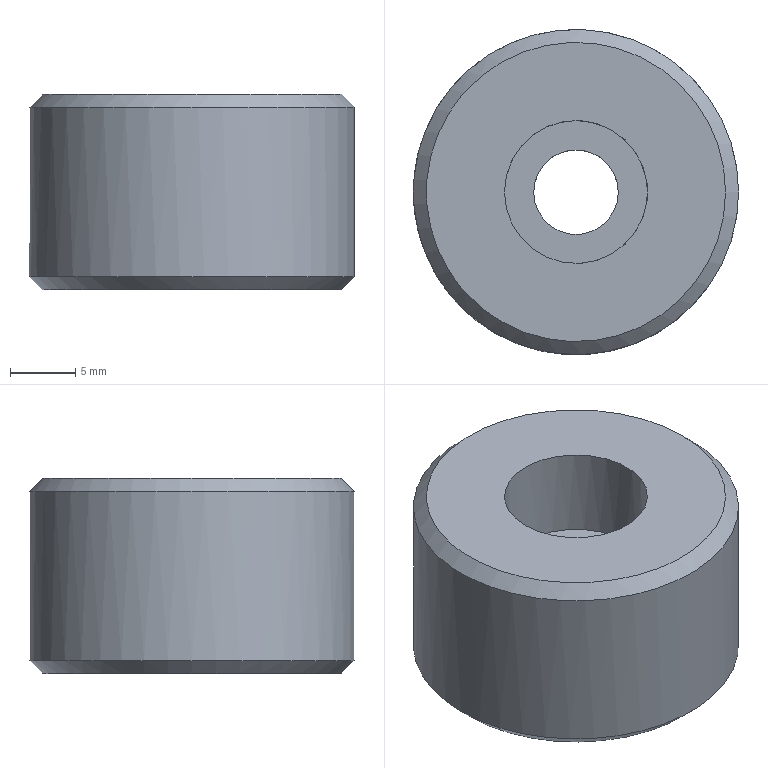Part | STEP file | lll_id122_x_t | 1 solid | 8 faces | box 25 x 25 x 15 mm | volume 6356 mm3 | plane 3 | cylinder 3 | cone 2 | commonest cylinder face diameters 6.5 x1 11 x1 25 x1
STEP:
#1=CARTESIAN_POINT('',(-28.5,-80.,-100.5));
#2=VERTEX_POINT('',#1);
#3=CARTESIAN_POINT('',(-40.,-80.,-100.5));
#4=DIRECTION('',(0.,0.,1.));
#5=DIRECTION('',(1.,0.,0.));
#6=AXIS2_PLACEMENT_3D('',#3,#4,#5);
#7=CIRCLE('',#6,11.5);
#8=EDGE_CURVE('',#2,#2,#7,.T.);
#9=ORIENTED_EDGE('',*,*,#8,.T.);
#10=EDGE_LOOP('',(#9));
#11=FACE_BOUND('',#10,.T.);
#12=CARTESIAN_POINT('',(-45.5,-80.,-100.5));
#13=VERTEX_POINT('',#12);
#14=CARTESIAN_POINT('',(-40.,-80.,-100.5));
#15=DIRECTION('',(0.,0.,-1.));
#16=DIRECTION('',(-1.,0.,0.));
#17=AXIS2_PLACEMENT_3D('',#14,#15,#16);
#18=CIRCLE('',#17,5.5);
#19=EDGE_CURVE('',#13,#13,#18,.T.);
#20=ORIENTED_EDGE('',*,*,#19,.T.);
#21=EDGE_LOOP('',(#20));
#22=FACE_BOUND('',#21,.T.);
#23=CARTESIAN_POINT('',(-40.,-80.,-100.5));
#24=DIRECTION('',(0.,0.,1.));
#25=DIRECTION('',(1.,0.,0.));
#26=AXIS2_PLACEMENT_3D('',#23,#24,#25);
#27=PLANE('',#26);
#28=ADVANCED_FACE('',(#11,#22),#27,.T.);
#29=CARTESIAN_POINT('',(-51.5,-80.,-115.5));
#30=VERTEX_POINT('',#29);
#31=CARTESIAN_POINT('',(-40.,-80.,-115.5));
#32=DIRECTION('',(0.,0.,-1.));
#33=DIRECTION('',(-1.,0.,0.));
#34=AXIS2_PLACEMENT_3D('',#31,#32,#33);
#35=CIRCLE('',#34,11.5);
#36=EDGE_CURVE('',#30,#30,#35,.T.);
#37=ORIENTED_EDGE('',*,*,#36,.T.);
#38=EDGE_LOOP('',(#37));
#39=FACE_BOUND('',#38,.T.);
#40=CARTESIAN_POINT('',(-36.75,-80.,-115.5));
#41=VERTEX_POINT('',#40);
#42=CARTESIAN_POINT('',(-40.,-80.,-115.5));
#43=DIRECTION('',(0.,0.,1.));
#44=DIRECTION('',(1.,0.,0.));
#45=AXIS2_PLACEMENT_3D('',#42,#43,#44);
#46=CIRCLE('',#45,3.25);
#47=EDGE_CURVE('',#41,#41,#46,.T.);
#48=ORIENTED_EDGE('',*,*,#47,.T.);
#49=EDGE_LOOP('',(#48));
#50=FACE_BOUND('',#49,.T.);
#51=CARTESIAN_POINT('',(-40.,-80.,-115.5));
#52=DIRECTION('',(0.,0.,-1.));
#53=DIRECTION('',(-1.,0.,0.));
#54=AXIS2_PLACEMENT_3D('',#51,#52,#53);
#55=PLANE('',#54);
#56=ADVANCED_FACE('',(#39,#50),#55,.T.);
#57=CARTESIAN_POINT('',(-52.5,-80.,-114.5));
#58=VERTEX_POINT('',#57);
#59=CARTESIAN_POINT('',(-40.,-80.,-114.5));
#60=DIRECTION('',(0.,0.,1.));
#61=DIRECTION('',(-1.,0.,0.));
#62=AXIS2_PLACEMENT_3D('',#59,#60,#61);
#63=CIRCLE('',#62,12.5);
#64=EDGE_CURVE('',#58,#58,#63,.T.);
#65=ORIENTED_EDGE('',*,*,#64,.T.);
#66=EDGE_LOOP('',(#65));
#67=FACE_BOUND('',#66,.T.);
#68=CARTESIAN_POINT('',(-27.5,-80.,-101.5));
#69=VERTEX_POINT('',#68);
#70=CARTESIAN_POINT('',(-40.,-80.,-101.5));
#71=DIRECTION('',(0.,0.,-1.));
#72=DIRECTION('',(1.,0.,0.));
#73=AXIS2_PLACEMENT_3D('',#70,#71,#72);
#74=CIRCLE('',#73,12.5);
#75=EDGE_CURVE('',#69,#69,#74,.T.);
#76=ORIENTED_EDGE('',*,*,#75,.T.);
#77=EDGE_LOOP('',(#76));
#78=FACE_BOUND('',#77,.T.);
#79=CARTESIAN_POINT('',(-40.,-80.,-115.5));
#80=DIRECTION('',(0.,0.,1.));
#81=DIRECTION('',(1.,0.,0.));
#82=AXIS2_PLACEMENT_3D('',#79,#80,#81);
#83=CYLINDRICAL_SURFACE('',#82,12.5);
#84=ADVANCED_FACE('',(#67,#78),#83,.T.);
#85=CARTESIAN_POINT('',(-43.25,-80.,-107.5));
#86=VERTEX_POINT('',#85);
#87=CARTESIAN_POINT('',(-40.,-80.,-107.5));
#88=DIRECTION('',(0.,0.,1.));
#89=DIRECTION('',(-1.,0.,0.));
#90=AXIS2_PLACEMENT_3D('',#87,#88,#89);
#91=CIRCLE('',#90,3.25);
#92=EDGE_CURVE('',#86,#86,#91,.T.);
#93=ORIENTED_EDGE('',*,*,#92,.T.);
#94=EDGE_LOOP('',(#93));
#95=FACE_BOUND('',#94,.T.);
#96=ORIENTED_EDGE('',*,*,#47,.F.);
#97=EDGE_LOOP('',(#96));
#98=FACE_BOUND('',#97,.T.);
#99=CARTESIAN_POINT('',(-40.,-80.,-100.5));
#100=DIRECTION('',(0.,0.,-1.));
#101=DIRECTION('',(-1.,0.,0.));
#102=AXIS2_PLACEMENT_3D('',#99,#100,#101);
#103=CYLINDRICAL_SURFACE('',#102,3.25);
#104=ADVANCED_FACE('',(#95,#98),#103,.F.);
#105=CARTESIAN_POINT('',(-34.5,-80.,-107.5));
#106=VERTEX_POINT('',#105);
#107=CARTESIAN_POINT('',(-40.,-80.,-107.5));
#108=DIRECTION('',(0.,0.,1.));
#109=DIRECTION('',(1.,0.,0.));
#110=AXIS2_PLACEMENT_3D('',#107,#108,#109);
#111=CIRCLE('',#110,5.5);
#112=EDGE_CURVE('',#106,#106,#111,.T.);
#113=ORIENTED_EDGE('',*,*,#112,.T.);
#114=EDGE_LOOP('',(#113));
#115=FACE_BOUND('',#114,.T.);
#116=ORIENTED_EDGE('',*,*,#92,.F.);
#117=EDGE_LOOP('',(#116));
#118=FACE_BOUND('',#117,.T.);
#119=CARTESIAN_POINT('',(-40.,-80.,-107.5));
#120=DIRECTION('',(0.,0.,-1.));
#121=DIRECTION('',(-1.,0.,0.));
#122=AXIS2_PLACEMENT_3D('',#119,#120,#121);
#123=PLANE('',#122);
#124=ADVANCED_FACE('',(#115,#118),#123,.F.);
#125=ORIENTED_EDGE('',*,*,#112,.F.);
#126=EDGE_LOOP('',(#125));
#127=FACE_BOUND('',#126,.T.);
#128=ORIENTED_EDGE('',*,*,#19,.F.);
#129=EDGE_LOOP('',(#128));
#130=FACE_BOUND('',#129,.T.);
#131=CARTESIAN_POINT('',(-40.,-80.,-100.5));
#132=DIRECTION('',(0.,0.,-1.));
#133=DIRECTION('',(-1.,0.,0.));
#134=AXIS2_PLACEMENT_3D('',#131,#132,#133);
#135=CYLINDRICAL_SURFACE('',#134,5.5);
#136=ADVANCED_FACE('',(#127,#130),#135,.F.);
#137=ORIENTED_EDGE('',*,*,#36,.F.);
#138=EDGE_LOOP('',(#137));
#139=FACE_BOUND('',#138,.T.);
#140=ORIENTED_EDGE('',*,*,#64,.F.);
#141=EDGE_LOOP('',(#140));
#142=FACE_BOUND('',#141,.T.);
#143=CARTESIAN_POINT('',(-40.,-80.,-114.5));
#144=DIRECTION('',(0.,0.,1.));
#145=DIRECTION('',(1.,0.,0.));
#146=AXIS2_PLACEMENT_3D('',#143,#144,#145);
#147=CONICAL_SURFACE('',#146,12.5,45.);
#148=ADVANCED_FACE('',(#139,#142),#147,.T.);
#149=ORIENTED_EDGE('',*,*,#8,.F.);
#150=EDGE_LOOP('',(#149));
#151=FACE_BOUND('',#150,.T.);
#152=ORIENTED_EDGE('',*,*,#75,.F.);
#153=EDGE_LOOP('',(#152));
#154=FACE_BOUND('',#153,.T.);
#155=CARTESIAN_POINT('',(-40.,-80.,-101.5));
#156=DIRECTION('',(0.,0.,-1.));
#157=DIRECTION('',(-1.,0.,0.));
#158=AXIS2_PLACEMENT_3D('',#155,#156,#157);
#159=CONICAL_SURFACE('',#158,12.5,45.);
#160=ADVANCED_FACE('',(#151,#154),#159,.T.);
#161=CLOSED_SHELL('',(#28,#56,#84,#104,#124,#136,#148,#160));
#162=MANIFOLD_SOLID_BREP('',#161);
#163=(LENGTH_UNIT()NAMED_UNIT(*)SI_UNIT(.MILLI.,.METRE.));
#164=UNCERTAINTY_MEASURE_WITH_UNIT(LENGTH_MEASURE(0.00002),#163,'','');
#165=(NAMED_UNIT(*)PLANE_ANGLE_UNIT()SI_UNIT($,.RADIAN.));
#166=PLANE_ANGLE_MEASURE_WITH_UNIT(PLANE_ANGLE_MEASURE(0.01745),#165);
#167=DIMENSIONAL_EXPONENTS(0.,0.,0.,0.,0.,0.,0.);
#168=(CONVERSION_BASED_UNIT('DEGREE',#166)NAMED_UNIT(#167)PLANE_ANGLE_UNIT());
#169=(NAMED_UNIT(*)SI_UNIT($,.STERADIAN.)SOLID_ANGLE_UNIT());
#170=(GEOMETRIC_REPRESENTATION_CONTEXT(3)GLOBAL_UNCERTAINTY_ASSIGNED_CONTEXT((#164))GLOBAL_UNIT_ASSIGNED_CONTEXT((#163,#168,#169))REPRESENTATION_CONTEXT('',''));
#171=ADVANCED_BREP_SHAPE_REPRESENTATION('',(#162),#170);